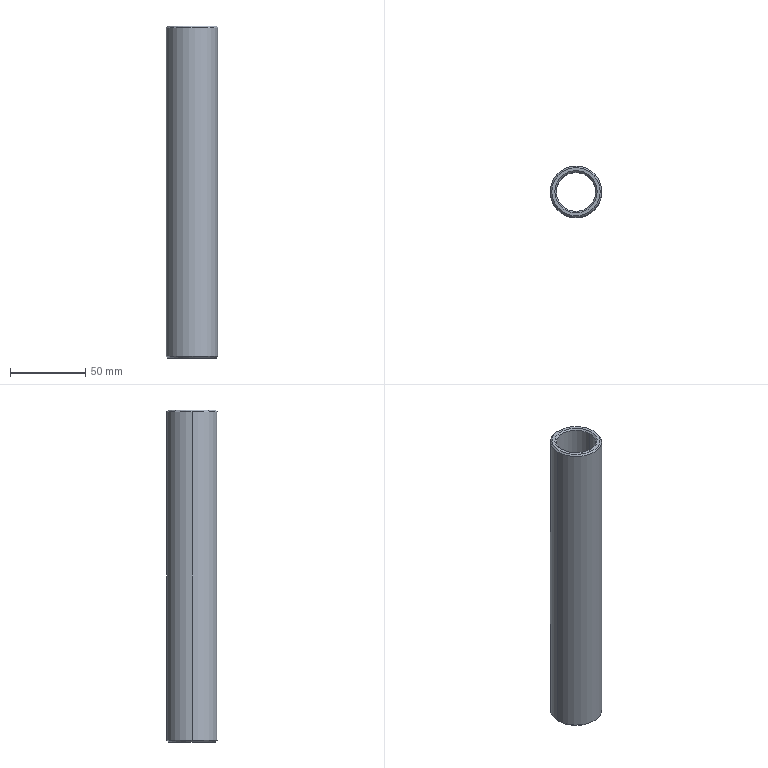Part | SolidWorks | features BaseBody 1 | 1 solid | 14 faces | box 34 x 34 x 220 mm | volume 82750 mm3 | cone 8 | cylinder 4 | plane 2 | commonest cylinder face diameters 26 x2 34 x2
STEP:
#1=CARTESIAN_POINT('',(13.,0.,-109.));
#2=VERTEX_POINT('',#1);
#3=CARTESIAN_POINT('',(14.,0.,-110.));
#4=VERTEX_POINT('',#3);
#5=CARTESIAN_POINT('',(14.,0.,-110.));
#6=DIRECTION('',(0.7071,0.,-0.7071));
#7=VECTOR('',#6,1000.);
#8=LINE('',#5,#7);
#9=EDGE_CURVE('',#2,#4,#8,.T.);
#10=ORIENTED_EDGE('',*,*,#9,.F.);
#11=CARTESIAN_POINT('',(-13.,0.,-109.));
#12=VERTEX_POINT('',#11);
#13=CARTESIAN_POINT('',(0.,0.,-109.));
#14=DIRECTION('',(0.,0.,-1.));
#15=DIRECTION('',(1.,0.,0.));
#16=AXIS2_PLACEMENT_3D('',#13,#14,#15);
#17=CIRCLE('',#16,13.);
#18=EDGE_CURVE('',#12,#2,#17,.T.);
#19=ORIENTED_EDGE('',*,*,#18,.F.);
#20=CARTESIAN_POINT('',(-14.,0.,-110.));
#21=VERTEX_POINT('',#20);
#22=CARTESIAN_POINT('',(-14.,0.,-110.));
#23=DIRECTION('',(-0.7071,0.,-0.7071));
#24=VECTOR('',#23,1000.);
#25=LINE('',#22,#24);
#26=EDGE_CURVE('',#12,#21,#25,.T.);
#27=ORIENTED_EDGE('',*,*,#26,.T.);
#28=CARTESIAN_POINT('',(0.,0.,-110.));
#29=DIRECTION('',(0.,0.,1.));
#30=DIRECTION('',(1.,0.,0.));
#31=AXIS2_PLACEMENT_3D('',#28,#29,#30);
#32=CIRCLE('',#31,14.);
#33=EDGE_CURVE('',#4,#21,#32,.T.);
#34=ORIENTED_EDGE('',*,*,#33,.F.);
#35=EDGE_LOOP('',(#10,#19,#27,#34));
#36=FACE_OUTER_BOUND('',#35,.T.);
#37=CARTESIAN_POINT('',(0.,0.,-110.));
#38=DIRECTION('',(0.,0.,-1.));
#39=DIRECTION('',(-1.,0.,0.));
#40=AXIS2_PLACEMENT_3D('',#37,#38,#39);
#41=CONICAL_SURFACE('',#40,14.,0.7854);
#42=ADVANCED_FACE('',(#36),#41,.F.);
#43=CARTESIAN_POINT('',(-16.,0.,-110.));
#44=VERTEX_POINT('',#43);
#45=CARTESIAN_POINT('',(-17.,0.,-109.));
#46=VERTEX_POINT('',#45);
#47=CARTESIAN_POINT('',(-17.,0.,-109.));
#48=DIRECTION('',(-0.7071,0.,0.7071));
#49=VECTOR('',#48,1000.);
#50=LINE('',#47,#49);
#51=EDGE_CURVE('',#44,#46,#50,.T.);
#52=ORIENTED_EDGE('',*,*,#51,.F.);
#53=CARTESIAN_POINT('',(16.,0.,-110.));
#54=VERTEX_POINT('',#53);
#55=CARTESIAN_POINT('',(0.,0.,-110.));
#56=DIRECTION('',(0.,0.,-1.));
#57=DIRECTION('',(1.,0.,0.));
#58=AXIS2_PLACEMENT_3D('',#55,#56,#57);
#59=CIRCLE('',#58,16.);
#60=EDGE_CURVE('',#54,#44,#59,.T.);
#61=ORIENTED_EDGE('',*,*,#60,.F.);
#62=CARTESIAN_POINT('',(17.,0.,-109.));
#63=VERTEX_POINT('',#62);
#64=CARTESIAN_POINT('',(17.,0.,-109.));
#65=DIRECTION('',(0.7071,0.,0.7071));
#66=VECTOR('',#65,1000.);
#67=LINE('',#64,#66);
#68=EDGE_CURVE('',#54,#63,#67,.T.);
#69=ORIENTED_EDGE('',*,*,#68,.T.);
#70=CARTESIAN_POINT('',(0.,0.,-109.));
#71=DIRECTION('',(0.,0.,1.));
#72=DIRECTION('',(1.,0.,0.));
#73=AXIS2_PLACEMENT_3D('',#70,#71,#72);
#74=CIRCLE('',#73,17.);
#75=EDGE_CURVE('',#46,#63,#74,.T.);
#76=ORIENTED_EDGE('',*,*,#75,.F.);
#77=EDGE_LOOP('',(#52,#61,#69,#76));
#78=FACE_OUTER_BOUND('',#77,.T.);
#79=CARTESIAN_POINT('',(0.,0.,-109.));
#80=DIRECTION('',(0.,0.,1.));
#81=DIRECTION('',(1.,0.,0.));
#82=AXIS2_PLACEMENT_3D('',#79,#80,#81);
#83=CONICAL_SURFACE('',#82,17.,0.7854);
#84=ADVANCED_FACE('',(#78),#83,.T.);
#85=CARTESIAN_POINT('',(-13.,0.,109.));
#86=VERTEX_POINT('',#85);
#87=CARTESIAN_POINT('',(-14.,0.,110.));
#88=VERTEX_POINT('',#87);
#89=CARTESIAN_POINT('',(-13.,0.,109.));
#90=DIRECTION('',(-0.7071,0.,0.7071));
#91=VECTOR('',#90,1000.);
#92=LINE('',#89,#91);
#93=EDGE_CURVE('',#86,#88,#92,.T.);
#94=ORIENTED_EDGE('',*,*,#93,.F.);
#95=CARTESIAN_POINT('',(13.,0.,109.));
#96=VERTEX_POINT('',#95);
#97=CARTESIAN_POINT('',(0.,0.,109.));
#98=DIRECTION('',(0.,0.,1.));
#99=DIRECTION('',(1.,0.,0.));
#100=AXIS2_PLACEMENT_3D('',#97,#98,#99);
#101=CIRCLE('',#100,13.);
#102=EDGE_CURVE('',#96,#86,#101,.T.);
#103=ORIENTED_EDGE('',*,*,#102,.F.);
#104=CARTESIAN_POINT('',(14.,0.,110.));
#105=VERTEX_POINT('',#104);
#106=CARTESIAN_POINT('',(13.,0.,109.));
#107=DIRECTION('',(0.7071,0.,0.7071));
#108=VECTOR('',#107,1000.);
#109=LINE('',#106,#108);
#110=EDGE_CURVE('',#96,#105,#109,.T.);
#111=ORIENTED_EDGE('',*,*,#110,.T.);
#112=CARTESIAN_POINT('',(0.,0.,110.));
#113=DIRECTION('',(0.,0.,-1.));
#114=DIRECTION('',(1.,0.,0.));
#115=AXIS2_PLACEMENT_3D('',#112,#113,#114);
#116=CIRCLE('',#115,14.);
#117=EDGE_CURVE('',#88,#105,#116,.T.);
#118=ORIENTED_EDGE('',*,*,#117,.F.);
#119=EDGE_LOOP('',(#94,#103,#111,#118));
#120=FACE_OUTER_BOUND('',#119,.T.);
#121=CARTESIAN_POINT('',(0.,0.,109.));
#122=DIRECTION('',(0.,0.,1.));
#123=DIRECTION('',(1.,0.,0.));
#124=AXIS2_PLACEMENT_3D('',#121,#122,#123);
#125=CONICAL_SURFACE('',#124,13.,0.7854);
#126=ADVANCED_FACE('',(#120),#125,.F.);
#127=CARTESIAN_POINT('',(16.,0.,110.));
#128=VERTEX_POINT('',#127);
#129=CARTESIAN_POINT('',(17.,0.,109.));
#130=VERTEX_POINT('',#129);
#131=CARTESIAN_POINT('',(16.,0.,110.));
#132=DIRECTION('',(0.7071,0.,-0.7071));
#133=VECTOR('',#132,1000.);
#134=LINE('',#131,#133);
#135=EDGE_CURVE('',#128,#130,#134,.T.);
#136=ORIENTED_EDGE('',*,*,#135,.F.);
#137=CARTESIAN_POINT('',(-16.,0.,110.));
#138=VERTEX_POINT('',#137);
#139=CARTESIAN_POINT('',(0.,0.,110.));
#140=DIRECTION('',(0.,0.,1.));
#141=DIRECTION('',(1.,0.,0.));
#142=AXIS2_PLACEMENT_3D('',#139,#140,#141);
#143=CIRCLE('',#142,16.);
#144=EDGE_CURVE('',#138,#128,#143,.T.);
#145=ORIENTED_EDGE('',*,*,#144,.F.);
#146=CARTESIAN_POINT('',(-17.,0.,109.));
#147=VERTEX_POINT('',#146);
#148=CARTESIAN_POINT('',(-16.,0.,110.));
#149=DIRECTION('',(-0.7071,0.,-0.7071));
#150=VECTOR('',#149,1000.);
#151=LINE('',#148,#150);
#152=EDGE_CURVE('',#138,#147,#151,.T.);
#153=ORIENTED_EDGE('',*,*,#152,.T.);
#154=CARTESIAN_POINT('',(0.,0.,109.));
#155=DIRECTION('',(0.,0.,-1.));
#156=DIRECTION('',(1.,0.,0.));
#157=AXIS2_PLACEMENT_3D('',#154,#155,#156);
#158=CIRCLE('',#157,17.);
#159=EDGE_CURVE('',#130,#147,#158,.T.);
#160=ORIENTED_EDGE('',*,*,#159,.F.);
#161=EDGE_LOOP('',(#136,#145,#153,#160));
#162=FACE_OUTER_BOUND('',#161,.T.);
#163=CARTESIAN_POINT('',(0.,0.,110.));
#164=DIRECTION('',(0.,0.,-1.));
#165=DIRECTION('',(-1.,0.,0.));
#166=AXIS2_PLACEMENT_3D('',#163,#164,#165);
#167=CONICAL_SURFACE('',#166,16.,0.7854);
#168=ADVANCED_FACE('',(#162),#167,.T.);
#169=CARTESIAN_POINT('',(-13.,0.,-110.));
#170=DIRECTION('',(0.,0.,1.));
#171=VECTOR('',#170,1000.);
#172=LINE('',#169,#171);
#173=EDGE_CURVE('',#12,#86,#172,.T.);
#174=ORIENTED_EDGE('',*,*,#173,.F.);
#175=ORIENTED_EDGE('',*,*,#18,.T.);
#176=CARTESIAN_POINT('',(13.,0.,-110.));
#177=DIRECTION('',(0.,0.,1.));
#178=VECTOR('',#177,1000.);
#179=LINE('',#176,#178);
#180=EDGE_CURVE('',#2,#96,#179,.T.);
#181=ORIENTED_EDGE('',*,*,#180,.T.);
#182=ORIENTED_EDGE('',*,*,#102,.T.);
#183=EDGE_LOOP('',(#174,#175,#181,#182));
#184=FACE_OUTER_BOUND('',#183,.T.);
#185=CARTESIAN_POINT('',(0.,0.,-110.));
#186=DIRECTION('',(0.,0.,1.));
#187=DIRECTION('',(1.,0.,0.));
#188=AXIS2_PLACEMENT_3D('',#185,#186,#187);
#189=CYLINDRICAL_SURFACE('',#188,13.);
#190=ADVANCED_FACE('',(#184),#189,.F.);
#191=CARTESIAN_POINT('',(0.,0.,110.));
#192=DIRECTION('',(0.,0.,-1.));
#193=DIRECTION('',(1.,0.,0.));
#194=AXIS2_PLACEMENT_3D('',#191,#192,#193);
#195=CIRCLE('',#194,14.);
#196=EDGE_CURVE('',#105,#88,#195,.T.);
#197=ORIENTED_EDGE('',*,*,#196,.T.);
#198=ORIENTED_EDGE('',*,*,#117,.T.);
#199=EDGE_LOOP('',(#197,#198));
#200=FACE_BOUND('',#199,.T.);
#201=ORIENTED_EDGE('',*,*,#144,.T.);
#202=CARTESIAN_POINT('',(0.,0.,110.));
#203=DIRECTION('',(0.,0.,1.));
#204=DIRECTION('',(1.,0.,0.));
#205=AXIS2_PLACEMENT_3D('',#202,#203,#204);
#206=CIRCLE('',#205,16.);
#207=EDGE_CURVE('',#128,#138,#206,.T.);
#208=ORIENTED_EDGE('',*,*,#207,.T.);
#209=EDGE_LOOP('',(#201,#208));
#210=FACE_OUTER_BOUND('',#209,.T.);
#211=CARTESIAN_POINT('',(0.,0.,110.));
#212=DIRECTION('',(0.,0.,1.));
#213=DIRECTION('',(1.,0.,0.));
#214=AXIS2_PLACEMENT_3D('',#211,#212,#213);
#215=PLANE('',#214);
#216=ADVANCED_FACE('',(#200,#210),#215,.T.);
#217=CARTESIAN_POINT('',(0.,0.,-110.));
#218=DIRECTION('',(0.,0.,1.));
#219=DIRECTION('',(1.,0.,0.));
#220=AXIS2_PLACEMENT_3D('',#217,#218,#219);
#221=CIRCLE('',#220,14.);
#222=EDGE_CURVE('',#21,#4,#221,.T.);
#223=ORIENTED_EDGE('',*,*,#222,.T.);
#224=ORIENTED_EDGE('',*,*,#33,.T.);
#225=EDGE_LOOP('',(#223,#224));
#226=FACE_BOUND('',#225,.T.);
#227=ORIENTED_EDGE('',*,*,#60,.T.);
#228=CARTESIAN_POINT('',(0.,0.,-110.));
#229=DIRECTION('',(0.,0.,-1.));
#230=DIRECTION('',(1.,0.,0.));
#231=AXIS2_PLACEMENT_3D('',#228,#229,#230);
#232=CIRCLE('',#231,16.);
#233=EDGE_CURVE('',#44,#54,#232,.T.);
#234=ORIENTED_EDGE('',*,*,#233,.T.);
#235=EDGE_LOOP('',(#227,#234));
#236=FACE_OUTER_BOUND('',#235,.T.);
#237=CARTESIAN_POINT('',(0.,0.,-110.));
#238=DIRECTION('',(0.,0.,1.));
#239=DIRECTION('',(1.,0.,0.));
#240=AXIS2_PLACEMENT_3D('',#237,#238,#239);
#241=PLANE('',#240);
#242=ADVANCED_FACE('',(#226,#236),#241,.F.);
#243=CARTESIAN_POINT('',(-17.,0.,-110.));
#244=DIRECTION('',(0.,0.,1.));
#245=VECTOR('',#244,1000.);
#246=LINE('',#243,#245);
#247=EDGE_CURVE('',#46,#147,#246,.T.);
#248=ORIENTED_EDGE('',*,*,#247,.F.);
#249=ORIENTED_EDGE('',*,*,#75,.T.);
#250=CARTESIAN_POINT('',(17.,0.,-110.));
#251=DIRECTION('',(0.,0.,1.));
#252=VECTOR('',#251,1000.);
#253=LINE('',#250,#252);
#254=EDGE_CURVE('',#63,#130,#253,.T.);
#255=ORIENTED_EDGE('',*,*,#254,.T.);
#256=ORIENTED_EDGE('',*,*,#159,.T.);
#257=EDGE_LOOP('',(#248,#249,#255,#256));
#258=FACE_OUTER_BOUND('',#257,.T.);
#259=CARTESIAN_POINT('',(0.,0.,-110.));
#260=DIRECTION('',(0.,0.,1.));
#261=DIRECTION('',(1.,0.,0.));
#262=AXIS2_PLACEMENT_3D('',#259,#260,#261);
#263=CYLINDRICAL_SURFACE('',#262,17.);
#264=ADVANCED_FACE('',(#258),#263,.T.);
#265=CARTESIAN_POINT('',(0.,0.,-109.));
#266=DIRECTION('',(0.,0.,1.));
#267=DIRECTION('',(1.,0.,0.));
#268=AXIS2_PLACEMENT_3D('',#265,#266,#267);
#269=CIRCLE('',#268,17.);
#270=EDGE_CURVE('',#63,#46,#269,.T.);
#271=ORIENTED_EDGE('',*,*,#270,.T.);
#272=ORIENTED_EDGE('',*,*,#247,.T.);
#273=CARTESIAN_POINT('',(0.,0.,109.));
#274=DIRECTION('',(0.,0.,-1.));
#275=DIRECTION('',(1.,0.,0.));
#276=AXIS2_PLACEMENT_3D('',#273,#274,#275);
#277=CIRCLE('',#276,17.);
#278=EDGE_CURVE('',#147,#130,#277,.T.);
#279=ORIENTED_EDGE('',*,*,#278,.T.);
#280=ORIENTED_EDGE('',*,*,#254,.F.);
#281=EDGE_LOOP('',(#271,#272,#279,#280));
#282=FACE_OUTER_BOUND('',#281,.T.);
#283=CARTESIAN_POINT('',(0.,0.,-110.));
#284=DIRECTION('',(0.,0.,1.));
#285=DIRECTION('',(1.,0.,0.));
#286=AXIS2_PLACEMENT_3D('',#283,#284,#285);
#287=CYLINDRICAL_SURFACE('',#286,17.);
#288=ADVANCED_FACE('',(#282),#287,.T.);
#289=CARTESIAN_POINT('',(0.,0.,-109.));
#290=DIRECTION('',(0.,0.,-1.));
#291=DIRECTION('',(1.,0.,0.));
#292=AXIS2_PLACEMENT_3D('',#289,#290,#291);
#293=CIRCLE('',#292,13.);
#294=EDGE_CURVE('',#2,#12,#293,.T.);
#295=ORIENTED_EDGE('',*,*,#294,.T.);
#296=ORIENTED_EDGE('',*,*,#173,.T.);
#297=CARTESIAN_POINT('',(0.,0.,109.));
#298=DIRECTION('',(0.,0.,1.));
#299=DIRECTION('',(1.,0.,0.));
#300=AXIS2_PLACEMENT_3D('',#297,#298,#299);
#301=CIRCLE('',#300,13.);
#302=EDGE_CURVE('',#86,#96,#301,.T.);
#303=ORIENTED_EDGE('',*,*,#302,.T.);
#304=ORIENTED_EDGE('',*,*,#180,.F.);
#305=EDGE_LOOP('',(#295,#296,#303,#304));
#306=FACE_OUTER_BOUND('',#305,.T.);
#307=CARTESIAN_POINT('',(0.,0.,-110.));
#308=DIRECTION('',(0.,0.,1.));
#309=DIRECTION('',(1.,0.,0.));
#310=AXIS2_PLACEMENT_3D('',#307,#308,#309);
#311=CYLINDRICAL_SURFACE('',#310,13.);
#312=ADVANCED_FACE('',(#306),#311,.F.);
#313=ORIENTED_EDGE('',*,*,#207,.F.);
#314=ORIENTED_EDGE('',*,*,#135,.T.);
#315=ORIENTED_EDGE('',*,*,#278,.F.);
#316=ORIENTED_EDGE('',*,*,#152,.F.);
#317=EDGE_LOOP('',(#313,#314,#315,#316));
#318=FACE_OUTER_BOUND('',#317,.T.);
#319=CARTESIAN_POINT('',(0.,0.,110.));
#320=DIRECTION('',(0.,0.,-1.));
#321=DIRECTION('',(-1.,0.,0.));
#322=AXIS2_PLACEMENT_3D('',#319,#320,#321);
#323=CONICAL_SURFACE('',#322,16.,0.7854);
#324=ADVANCED_FACE('',(#318),#323,.T.);
#325=ORIENTED_EDGE('',*,*,#302,.F.);
#326=ORIENTED_EDGE('',*,*,#93,.T.);
#327=ORIENTED_EDGE('',*,*,#196,.F.);
#328=ORIENTED_EDGE('',*,*,#110,.F.);
#329=EDGE_LOOP('',(#325,#326,#327,#328));
#330=FACE_OUTER_BOUND('',#329,.T.);
#331=CARTESIAN_POINT('',(0.,0.,109.));
#332=DIRECTION('',(0.,0.,1.));
#333=DIRECTION('',(1.,0.,0.));
#334=AXIS2_PLACEMENT_3D('',#331,#332,#333);
#335=CONICAL_SURFACE('',#334,13.,0.7854);
#336=ADVANCED_FACE('',(#330),#335,.F.);
#337=ORIENTED_EDGE('',*,*,#233,.F.);
#338=ORIENTED_EDGE('',*,*,#51,.T.);
#339=ORIENTED_EDGE('',*,*,#270,.F.);
#340=ORIENTED_EDGE('',*,*,#68,.F.);
#341=EDGE_LOOP('',(#337,#338,#339,#340));
#342=FACE_OUTER_BOUND('',#341,.T.);
#343=CARTESIAN_POINT('',(0.,0.,-109.));
#344=DIRECTION('',(0.,0.,1.));
#345=DIRECTION('',(1.,0.,0.));
#346=AXIS2_PLACEMENT_3D('',#343,#344,#345);
#347=CONICAL_SURFACE('',#346,17.,0.7854);
#348=ADVANCED_FACE('',(#342),#347,.T.);
#349=ORIENTED_EDGE('',*,*,#294,.F.);
#350=ORIENTED_EDGE('',*,*,#9,.T.);
#351=ORIENTED_EDGE('',*,*,#222,.F.);
#352=ORIENTED_EDGE('',*,*,#26,.F.);
#353=EDGE_LOOP('',(#349,#350,#351,#352));
#354=FACE_OUTER_BOUND('',#353,.T.);
#355=CARTESIAN_POINT('',(0.,0.,-110.));
#356=DIRECTION('',(0.,0.,-1.));
#357=DIRECTION('',(-1.,0.,0.));
#358=AXIS2_PLACEMENT_3D('',#355,#356,#357);
#359=CONICAL_SURFACE('',#358,14.,0.7854);
#360=ADVANCED_FACE('',(#354),#359,.F.);
#361=CLOSED_SHELL('',(#42,#84,#126,#168,#190,#216,#242,#264,#288,#312,#324,#336,#348,#360));
#362=MANIFOLD_SOLID_BREP('',#361);
#363=CARTESIAN_POINT('',(0.,0.,0.));
#364=DIRECTION('',(0.,0.,1.));
#365=DIRECTION('',(1.,0.,0.));
#366=AXIS2_PLACEMENT_3D('',#363,#364,#365);
#367=(LENGTH_UNIT()NAMED_UNIT(*)SI_UNIT(.MILLI.,.METRE.));
#368=UNCERTAINTY_MEASURE_WITH_UNIT(LENGTH_MEASURE(0.00001),#367,'','');
#369=(NAMED_UNIT(*)PLANE_ANGLE_UNIT()SI_UNIT($,.RADIAN.));
#370=(NAMED_UNIT(*)SI_UNIT($,.STERADIAN.)SOLID_ANGLE_UNIT());
#371=(GEOMETRIC_REPRESENTATION_CONTEXT(3)GLOBAL_UNCERTAINTY_ASSIGNED_CONTEXT((#368))GLOBAL_UNIT_ASSIGNED_CONTEXT((#367,#369,#370))REPRESENTATION_CONTEXT('',''));
#372=ADVANCED_BREP_SHAPE_REPRESENTATION('',(#362,#366),#371);